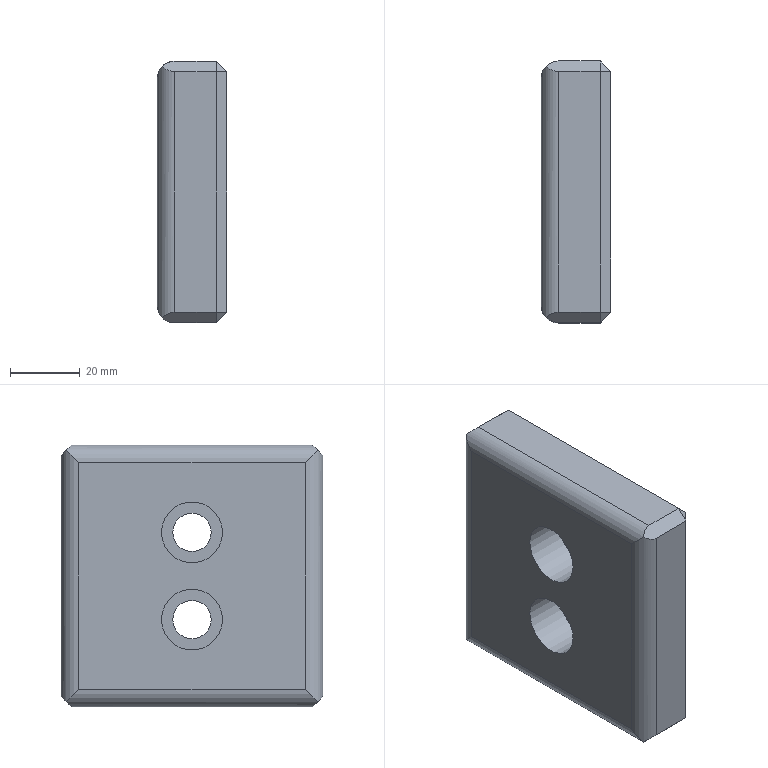Part | NX | features MAIN_BODY 2 | 1 solid | 28 faces | box 20 x 75 x 75 mm | volume 102061 mm3 | plane 20 | cylinder 8 | commonest cylinder face diameters 10 x4 11 x2 17.5 x2
STEP:
#1=CARTESIAN_POINT('',(-393.,34.5,70.));
#2=VERTEX_POINT('',#1);
#3=CARTESIAN_POINT('',(-405.,34.5,70.));
#4=VERTEX_POINT('',#3);
#5=CARTESIAN_POINT('',(-410.,34.5,70.));
#6=DIRECTION('',(-1.,0.,0.));
#7=VECTOR('',#6,1000.);
#8=LINE('',#5,#7);
#9=EDGE_CURVE('',#2,#4,#8,.T.);
#10=ORIENTED_EDGE('',*,*,#9,.T.);
#11=CARTESIAN_POINT('',(-405.,-34.5,70.));
#12=VERTEX_POINT('',#11);
#13=CARTESIAN_POINT('',(-405.,-34.5,70.));
#14=DIRECTION('',(0.,-1.,0.));
#15=VECTOR('',#14,1000.);
#16=LINE('',#13,#15);
#17=EDGE_CURVE('',#4,#12,#16,.T.);
#18=ORIENTED_EDGE('',*,*,#17,.T.);
#19=CARTESIAN_POINT('',(-393.,-34.5,70.));
#20=VERTEX_POINT('',#19);
#21=CARTESIAN_POINT('',(-410.,-34.5,70.));
#22=DIRECTION('',(1.,0.,0.));
#23=VECTOR('',#22,1000.);
#24=LINE('',#21,#23);
#25=EDGE_CURVE('',#12,#20,#24,.T.);
#26=ORIENTED_EDGE('',*,*,#25,.T.);
#27=CARTESIAN_POINT('',(-393.,37.5,70.));
#28=DIRECTION('',(0.,1.,0.));
#29=VECTOR('',#28,1000.);
#30=LINE('',#27,#29);
#31=EDGE_CURVE('',#20,#2,#30,.T.);
#32=ORIENTED_EDGE('',*,*,#31,.T.);
#33=EDGE_LOOP('',(#10,#18,#26,#32));
#34=FACE_BOUND('',#33,.T.);
#35=CARTESIAN_POINT('',(-410.,37.5,70.));
#36=DIRECTION('',(0.,0.,1.));
#37=DIRECTION('',(0.,1.,0.));
#38=AXIS2_PLACEMENT_3D('',#35,#36,#37);
#39=PLANE('',#38);
#40=ADVANCED_FACE('',(#34),#39,.T.);
#41=CARTESIAN_POINT('',(-393.,-37.5,67.));
#42=VERTEX_POINT('',#41);
#43=CARTESIAN_POINT('',(-405.,-37.5,67.));
#44=VERTEX_POINT('',#43);
#45=CARTESIAN_POINT('',(-410.,-37.5,67.));
#46=DIRECTION('',(-1.,0.,0.));
#47=VECTOR('',#46,1000.);
#48=LINE('',#45,#47);
#49=EDGE_CURVE('',#42,#44,#48,.T.);
#50=ORIENTED_EDGE('',*,*,#49,.T.);
#51=CARTESIAN_POINT('',(-405.,-37.5,-2.));
#52=VERTEX_POINT('',#51);
#53=CARTESIAN_POINT('',(-405.,-37.5,-2.));
#54=DIRECTION('',(0.,0.,-1.));
#55=VECTOR('',#54,1000.);
#56=LINE('',#53,#55);
#57=EDGE_CURVE('',#44,#52,#56,.T.);
#58=ORIENTED_EDGE('',*,*,#57,.T.);
#59=CARTESIAN_POINT('',(-393.,-37.5,-2.));
#60=VERTEX_POINT('',#59);
#61=CARTESIAN_POINT('',(-410.,-37.5,-2.));
#62=DIRECTION('',(1.,0.,0.));
#63=VECTOR('',#62,1000.);
#64=LINE('',#61,#63);
#65=EDGE_CURVE('',#52,#60,#64,.T.);
#66=ORIENTED_EDGE('',*,*,#65,.T.);
#67=CARTESIAN_POINT('',(-393.,-37.5,70.));
#68=DIRECTION('',(0.,0.,1.));
#69=VECTOR('',#68,1000.);
#70=LINE('',#67,#69);
#71=EDGE_CURVE('',#60,#42,#70,.T.);
#72=ORIENTED_EDGE('',*,*,#71,.T.);
#73=EDGE_LOOP('',(#50,#58,#66,#72));
#74=FACE_BOUND('',#73,.T.);
#75=CARTESIAN_POINT('',(-410.,-37.5,70.));
#76=DIRECTION('',(0.,-1.,0.));
#77=DIRECTION('',(0.,0.,1.));
#78=AXIS2_PLACEMENT_3D('',#75,#76,#77);
#79=PLANE('',#78);
#80=ADVANCED_FACE('',(#74),#79,.T.);
#81=CARTESIAN_POINT('',(-393.,-34.5,-5.));
#82=VERTEX_POINT('',#81);
#83=CARTESIAN_POINT('',(-405.,-34.5,-5.));
#84=VERTEX_POINT('',#83);
#85=CARTESIAN_POINT('',(-410.,-34.5,-5.));
#86=DIRECTION('',(-1.,0.,0.));
#87=VECTOR('',#86,1000.);
#88=LINE('',#85,#87);
#89=EDGE_CURVE('',#82,#84,#88,.T.);
#90=ORIENTED_EDGE('',*,*,#89,.T.);
#91=CARTESIAN_POINT('',(-405.,34.5,-5.));
#92=VERTEX_POINT('',#91);
#93=CARTESIAN_POINT('',(-405.,34.5,-5.));
#94=DIRECTION('',(0.,1.,0.));
#95=VECTOR('',#94,1000.);
#96=LINE('',#93,#95);
#97=EDGE_CURVE('',#84,#92,#96,.T.);
#98=ORIENTED_EDGE('',*,*,#97,.T.);
#99=CARTESIAN_POINT('',(-393.,34.5,-5.));
#100=VERTEX_POINT('',#99);
#101=CARTESIAN_POINT('',(-410.,34.5,-5.));
#102=DIRECTION('',(1.,0.,0.));
#103=VECTOR('',#102,1000.);
#104=LINE('',#101,#103);
#105=EDGE_CURVE('',#92,#100,#104,.T.);
#106=ORIENTED_EDGE('',*,*,#105,.T.);
#107=CARTESIAN_POINT('',(-393.,-37.5,-5.));
#108=DIRECTION('',(0.,-1.,0.));
#109=VECTOR('',#108,1000.);
#110=LINE('',#107,#109);
#111=EDGE_CURVE('',#100,#82,#110,.T.);
#112=ORIENTED_EDGE('',*,*,#111,.T.);
#113=EDGE_LOOP('',(#90,#98,#106,#112));
#114=FACE_BOUND('',#113,.T.);
#115=CARTESIAN_POINT('',(-410.,-37.5,-5.));
#116=DIRECTION('',(0.,0.,-1.));
#117=DIRECTION('',(-1.,0.,0.));
#118=AXIS2_PLACEMENT_3D('',#115,#116,#117);
#119=PLANE('',#118);
#120=ADVANCED_FACE('',(#114),#119,.T.);
#121=CARTESIAN_POINT('',(-393.,37.5,-2.));
#122=VERTEX_POINT('',#121);
#123=CARTESIAN_POINT('',(-405.,37.5,-2.));
#124=VERTEX_POINT('',#123);
#125=CARTESIAN_POINT('',(-410.,37.5,-2.));
#126=DIRECTION('',(-1.,0.,0.));
#127=VECTOR('',#126,1000.);
#128=LINE('',#125,#127);
#129=EDGE_CURVE('',#122,#124,#128,.T.);
#130=ORIENTED_EDGE('',*,*,#129,.T.);
#131=CARTESIAN_POINT('',(-405.,37.5,67.));
#132=VERTEX_POINT('',#131);
#133=CARTESIAN_POINT('',(-405.,37.5,67.));
#134=DIRECTION('',(0.,0.,1.));
#135=VECTOR('',#134,1000.);
#136=LINE('',#133,#135);
#137=EDGE_CURVE('',#124,#132,#136,.T.);
#138=ORIENTED_EDGE('',*,*,#137,.T.);
#139=CARTESIAN_POINT('',(-393.,37.5,67.));
#140=VERTEX_POINT('',#139);
#141=CARTESIAN_POINT('',(-410.,37.5,67.));
#142=DIRECTION('',(1.,0.,0.));
#143=VECTOR('',#142,1000.);
#144=LINE('',#141,#143);
#145=EDGE_CURVE('',#132,#140,#144,.T.);
#146=ORIENTED_EDGE('',*,*,#145,.T.);
#147=CARTESIAN_POINT('',(-393.,37.5,-5.));
#148=DIRECTION('',(0.,0.,-1.));
#149=VECTOR('',#148,1000.);
#150=LINE('',#147,#149);
#151=EDGE_CURVE('',#140,#122,#150,.T.);
#152=ORIENTED_EDGE('',*,*,#151,.T.);
#153=EDGE_LOOP('',(#130,#138,#146,#152));
#154=FACE_BOUND('',#153,.T.);
#155=CARTESIAN_POINT('',(-410.,37.5,-5.));
#156=DIRECTION('',(0.,1.,0.));
#157=DIRECTION('',(0.,0.,-1.));
#158=AXIS2_PLACEMENT_3D('',#155,#156,#157);
#159=PLANE('',#158);
#160=ADVANCED_FACE('',(#154),#159,.T.);
#161=CARTESIAN_POINT('',(-410.,-32.5,0.));
#162=VERTEX_POINT('',#161);
#163=CARTESIAN_POINT('',(-410.,-32.5,65.));
#164=VERTEX_POINT('',#163);
#165=CARTESIAN_POINT('',(-410.,-32.5,67.));
#166=DIRECTION('',(0.,0.,-1.));
#167=VECTOR('',#166,1000.);
#168=LINE('',#165,#167);
#169=EDGE_CURVE('',#162,#164,#168,.F.);
#170=ORIENTED_EDGE('',*,*,#169,.T.);
#171=CARTESIAN_POINT('',(-410.,32.5,65.));
#172=VERTEX_POINT('',#171);
#173=CARTESIAN_POINT('',(-410.,34.5,65.));
#174=DIRECTION('',(0.,-1.,0.));
#175=VECTOR('',#174,1000.);
#176=LINE('',#173,#175);
#177=EDGE_CURVE('',#164,#172,#176,.F.);
#178=ORIENTED_EDGE('',*,*,#177,.T.);
#179=CARTESIAN_POINT('',(-410.,32.5,0.));
#180=VERTEX_POINT('',#179);
#181=CARTESIAN_POINT('',(-410.,32.5,-2.));
#182=DIRECTION('',(0.,0.,1.));
#183=VECTOR('',#182,1000.);
#184=LINE('',#181,#183);
#185=EDGE_CURVE('',#172,#180,#184,.F.);
#186=ORIENTED_EDGE('',*,*,#185,.T.);
#187=CARTESIAN_POINT('',(-410.,-34.5,0.));
#188=DIRECTION('',(0.,1.,0.));
#189=VECTOR('',#188,1000.);
#190=LINE('',#187,#189);
#191=EDGE_CURVE('',#180,#162,#190,.F.);
#192=ORIENTED_EDGE('',*,*,#191,.T.);
#193=EDGE_LOOP('',(#170,#178,#186,#192));
#194=FACE_BOUND('',#193,.T.);
#195=CARTESIAN_POINT('',(-410.,-8.75,20.));
#196=VERTEX_POINT('',#195);
#197=CARTESIAN_POINT('',(-410.,0.,20.));
#198=DIRECTION('',(1.,0.,0.));
#199=DIRECTION('',(0.,-1.,0.));
#200=AXIS2_PLACEMENT_3D('',#197,#198,#199);
#201=CIRCLE('',#200,8.75);
#202=EDGE_CURVE('',#196,#196,#201,.T.);
#203=ORIENTED_EDGE('',*,*,#202,.T.);
#204=EDGE_LOOP('',(#203));
#205=FACE_BOUND('',#204,.T.);
#206=CARTESIAN_POINT('',(-410.,-8.75,45.));
#207=VERTEX_POINT('',#206);
#208=CARTESIAN_POINT('',(-410.,0.,45.));
#209=DIRECTION('',(1.,0.,0.));
#210=DIRECTION('',(0.,-1.,0.));
#211=AXIS2_PLACEMENT_3D('',#208,#209,#210);
#212=CIRCLE('',#211,8.75);
#213=EDGE_CURVE('',#207,#207,#212,.T.);
#214=ORIENTED_EDGE('',*,*,#213,.T.);
#215=EDGE_LOOP('',(#214));
#216=FACE_BOUND('',#215,.T.);
#217=CARTESIAN_POINT('',(-410.,-37.5,70.));
#218=DIRECTION('',(1.,0.,0.));
#219=DIRECTION('',(0.,-1.,0.));
#220=AXIS2_PLACEMENT_3D('',#217,#218,#219);
#221=PLANE('',#220);
#222=ADVANCED_FACE('',(#194,#205,#216),#221,.F.);
#223=CARTESIAN_POINT('',(-390.,34.5,67.));
#224=VERTEX_POINT('',#223);
#225=CARTESIAN_POINT('',(-390.,-34.5,67.));
#226=VERTEX_POINT('',#225);
#227=CARTESIAN_POINT('',(-390.,-37.5,67.));
#228=DIRECTION('',(0.,-1.,0.));
#229=VECTOR('',#228,1000.);
#230=LINE('',#227,#229);
#231=EDGE_CURVE('',#224,#226,#230,.T.);
#232=ORIENTED_EDGE('',*,*,#231,.T.);
#233=CARTESIAN_POINT('',(-390.,-34.5,-2.));
#234=VERTEX_POINT('',#233);
#235=CARTESIAN_POINT('',(-390.,-34.5,70.));
#236=DIRECTION('',(0.,0.,-1.));
#237=VECTOR('',#236,1000.);
#238=LINE('',#235,#237);
#239=EDGE_CURVE('',#226,#234,#238,.T.);
#240=ORIENTED_EDGE('',*,*,#239,.T.);
#241=CARTESIAN_POINT('',(-390.,34.5,-2.));
#242=VERTEX_POINT('',#241);
#243=CARTESIAN_POINT('',(-390.,-37.5,-2.));
#244=DIRECTION('',(0.,1.,0.));
#245=VECTOR('',#244,1000.);
#246=LINE('',#243,#245);
#247=EDGE_CURVE('',#234,#242,#246,.T.);
#248=ORIENTED_EDGE('',*,*,#247,.T.);
#249=CARTESIAN_POINT('',(-390.,34.5,70.));
#250=DIRECTION('',(0.,0.,1.));
#251=VECTOR('',#250,1000.);
#252=LINE('',#249,#251);
#253=EDGE_CURVE('',#242,#224,#252,.T.);
#254=ORIENTED_EDGE('',*,*,#253,.T.);
#255=EDGE_LOOP('',(#232,#240,#248,#254));
#256=FACE_BOUND('',#255,.T.);
#257=CARTESIAN_POINT('',(-390.,-5.5,20.));
#258=VERTEX_POINT('',#257);
#259=CARTESIAN_POINT('',(-390.,0.,20.));
#260=DIRECTION('',(1.,0.,0.));
#261=DIRECTION('',(0.,-1.,0.));
#262=AXIS2_PLACEMENT_3D('',#259,#260,#261);
#263=CIRCLE('',#262,5.5);
#264=EDGE_CURVE('',#258,#258,#263,.T.);
#265=ORIENTED_EDGE('',*,*,#264,.F.);
#266=EDGE_LOOP('',(#265));
#267=FACE_BOUND('',#266,.T.);
#268=CARTESIAN_POINT('',(-390.,-5.5,45.));
#269=VERTEX_POINT('',#268);
#270=CARTESIAN_POINT('',(-390.,0.,45.));
#271=DIRECTION('',(1.,0.,0.));
#272=DIRECTION('',(0.,-1.,0.));
#273=AXIS2_PLACEMENT_3D('',#270,#271,#272);
#274=CIRCLE('',#273,5.5);
#275=EDGE_CURVE('',#269,#269,#274,.T.);
#276=ORIENTED_EDGE('',*,*,#275,.F.);
#277=EDGE_LOOP('',(#276));
#278=FACE_BOUND('',#277,.T.);
#279=CARTESIAN_POINT('',(-390.,-37.5,70.));
#280=DIRECTION('',(1.,0.,0.));
#281=DIRECTION('',(0.,-1.,0.));
#282=AXIS2_PLACEMENT_3D('',#279,#280,#281);
#283=PLANE('',#282);
#284=ADVANCED_FACE('',(#256,#267,#278),#283,.T.);
#285=ORIENTED_EDGE('',*,*,#275,.T.);
#286=EDGE_LOOP('',(#285));
#287=FACE_BOUND('',#286,.T.);
#288=CARTESIAN_POINT('',(-398.,-5.5,45.));
#289=VERTEX_POINT('',#288);
#290=CARTESIAN_POINT('',(-398.,0.,45.));
#291=DIRECTION('',(1.,0.,0.));
#292=DIRECTION('',(0.,-1.,0.));
#293=AXIS2_PLACEMENT_3D('',#290,#291,#292);
#294=CIRCLE('',#293,5.5);
#295=EDGE_CURVE('',#289,#289,#294,.T.);
#296=ORIENTED_EDGE('',*,*,#295,.F.);
#297=EDGE_LOOP('',(#296));
#298=FACE_BOUND('',#297,.T.);
#299=CARTESIAN_POINT('',(-360.,0.,45.));
#300=DIRECTION('',(1.,0.,0.));
#301=DIRECTION('',(0.,-1.,0.));
#302=AXIS2_PLACEMENT_3D('',#299,#300,#301);
#303=CYLINDRICAL_SURFACE('',#302,5.5);
#304=ADVANCED_FACE('',(#287,#298),#303,.F.);
#305=ORIENTED_EDGE('',*,*,#295,.T.);
#306=EDGE_LOOP('',(#305));
#307=FACE_BOUND('',#306,.T.);
#308=CARTESIAN_POINT('',(-398.,-8.75,45.));
#309=VERTEX_POINT('',#308);
#310=CARTESIAN_POINT('',(-398.,0.,45.));
#311=DIRECTION('',(1.,0.,0.));
#312=DIRECTION('',(0.,-1.,0.));
#313=AXIS2_PLACEMENT_3D('',#310,#311,#312);
#314=CIRCLE('',#313,8.75);
#315=EDGE_CURVE('',#309,#309,#314,.T.);
#316=ORIENTED_EDGE('',*,*,#315,.F.);
#317=EDGE_LOOP('',(#316));
#318=FACE_BOUND('',#317,.T.);
#319=CARTESIAN_POINT('',(-398.,0.,45.));
#320=DIRECTION('',(1.,0.,0.));
#321=DIRECTION('',(0.,-1.,0.));
#322=AXIS2_PLACEMENT_3D('',#319,#320,#321);
#323=PLANE('',#322);
#324=ADVANCED_FACE('',(#307,#318),#323,.F.);
#325=ORIENTED_EDGE('',*,*,#315,.T.);
#326=EDGE_LOOP('',(#325));
#327=FACE_BOUND('',#326,.T.);
#328=ORIENTED_EDGE('',*,*,#213,.F.);
#329=EDGE_LOOP('',(#328));
#330=FACE_BOUND('',#329,.T.);
#331=CARTESIAN_POINT('',(-410.,0.,45.));
#332=DIRECTION('',(1.,0.,0.));
#333=DIRECTION('',(0.,-1.,0.));
#334=AXIS2_PLACEMENT_3D('',#331,#332,#333);
#335=CYLINDRICAL_SURFACE('',#334,8.75);
#336=ADVANCED_FACE('',(#327,#330),#335,.F.);
#337=ORIENTED_EDGE('',*,*,#264,.T.);
#338=EDGE_LOOP('',(#337));
#339=FACE_BOUND('',#338,.T.);
#340=CARTESIAN_POINT('',(-398.,-5.5,20.));
#341=VERTEX_POINT('',#340);
#342=CARTESIAN_POINT('',(-398.,0.,20.));
#343=DIRECTION('',(1.,0.,0.));
#344=DIRECTION('',(0.,-1.,0.));
#345=AXIS2_PLACEMENT_3D('',#342,#343,#344);
#346=CIRCLE('',#345,5.5);
#347=EDGE_CURVE('',#341,#341,#346,.T.);
#348=ORIENTED_EDGE('',*,*,#347,.F.);
#349=EDGE_LOOP('',(#348));
#350=FACE_BOUND('',#349,.T.);
#351=CARTESIAN_POINT('',(-360.,0.,20.));
#352=DIRECTION('',(1.,0.,0.));
#353=DIRECTION('',(0.,-1.,0.));
#354=AXIS2_PLACEMENT_3D('',#351,#352,#353);
#355=CYLINDRICAL_SURFACE('',#354,5.5);
#356=ADVANCED_FACE('',(#339,#350),#355,.F.);
#357=ORIENTED_EDGE('',*,*,#347,.T.);
#358=EDGE_LOOP('',(#357));
#359=FACE_BOUND('',#358,.T.);
#360=CARTESIAN_POINT('',(-398.,-8.75,20.));
#361=VERTEX_POINT('',#360);
#362=CARTESIAN_POINT('',(-398.,0.,20.));
#363=DIRECTION('',(1.,0.,0.));
#364=DIRECTION('',(0.,-1.,0.));
#365=AXIS2_PLACEMENT_3D('',#362,#363,#364);
#366=CIRCLE('',#365,8.75);
#367=EDGE_CURVE('',#361,#361,#366,.T.);
#368=ORIENTED_EDGE('',*,*,#367,.F.);
#369=EDGE_LOOP('',(#368));
#370=FACE_BOUND('',#369,.T.);
#371=CARTESIAN_POINT('',(-398.,0.,20.));
#372=DIRECTION('',(1.,0.,0.));
#373=DIRECTION('',(0.,-1.,0.));
#374=AXIS2_PLACEMENT_3D('',#371,#372,#373);
#375=PLANE('',#374);
#376=ADVANCED_FACE('',(#359,#370),#375,.F.);
#377=ORIENTED_EDGE('',*,*,#367,.T.);
#378=EDGE_LOOP('',(#377));
#379=FACE_BOUND('',#378,.T.);
#380=ORIENTED_EDGE('',*,*,#202,.F.);
#381=EDGE_LOOP('',(#380));
#382=FACE_BOUND('',#381,.T.);
#383=CARTESIAN_POINT('',(-410.,0.,20.));
#384=DIRECTION('',(1.,0.,0.));
#385=DIRECTION('',(0.,-1.,0.));
#386=AXIS2_PLACEMENT_3D('',#383,#384,#385);
#387=CYLINDRICAL_SURFACE('',#386,8.75);
#388=ADVANCED_FACE('',(#379,#382),#387,.F.);
#389=CARTESIAN_POINT('',(-408.571,36.,68.5));
#390=VERTEX_POINT('',#389);
#391=CARTESIAN_POINT('',(-405.,32.5,72.));
#392=DIRECTION('',(0.,-0.7071,-0.7071));
#393=DIRECTION('',(0.,0.7071,-0.7071));
#394=AXIS2_PLACEMENT_3D('',#391,#392,#393);
#395=ELLIPSE('',#394,7.071,5.);
#396=EDGE_CURVE('',#132,#390,#395,.F.);
#397=ORIENTED_EDGE('',*,*,#396,.T.);
#398=CARTESIAN_POINT('',(-405.,39.5,65.));
#399=DIRECTION('',(0.,-0.7071,-0.7071));
#400=DIRECTION('',(0.,0.7071,-0.7071));
#401=AXIS2_PLACEMENT_3D('',#398,#399,#400);
#402=ELLIPSE('',#401,7.071,5.);
#403=EDGE_CURVE('',#390,#4,#402,.F.);
#404=ORIENTED_EDGE('',*,*,#403,.T.);
#405=ORIENTED_EDGE('',*,*,#9,.F.);
#406=CARTESIAN_POINT('',(-393.,36.,68.5));
#407=DIRECTION('',(0.,0.7071,-0.7071));
#408=VECTOR('',#407,1000.);
#409=LINE('',#406,#408);
#410=EDGE_CURVE('',#140,#2,#409,.F.);
#411=ORIENTED_EDGE('',*,*,#410,.F.);
#412=ORIENTED_EDGE('',*,*,#145,.F.);
#413=EDGE_LOOP('',(#397,#404,#405,#411,#412));
#414=FACE_BOUND('',#413,.T.);
#415=CARTESIAN_POINT('',(-410.,37.5,67.));
#416=DIRECTION('',(0.,-0.7071,-0.7071));
#417=DIRECTION('',(0.,-0.7071,0.7071));
#418=AXIS2_PLACEMENT_3D('',#415,#416,#417);
#419=PLANE('',#418);
#420=ADVANCED_FACE('',(#414),#419,.F.);
#421=CARTESIAN_POINT('',(-390.,34.5,-2.));
#422=DIRECTION('',(-0.7071,0.7071,0.));
#423=VECTOR('',#422,1000.);
#424=LINE('',#421,#423);
#425=EDGE_CURVE('',#122,#242,#424,.F.);
#426=ORIENTED_EDGE('',*,*,#425,.F.);
#427=ORIENTED_EDGE('',*,*,#151,.F.);
#428=CARTESIAN_POINT('',(-390.,34.5,67.));
#429=DIRECTION('',(0.7071,-0.7071,0.));
#430=VECTOR('',#429,1000.);
#431=LINE('',#428,#430);
#432=EDGE_CURVE('',#224,#140,#431,.F.);
#433=ORIENTED_EDGE('',*,*,#432,.F.);
#434=ORIENTED_EDGE('',*,*,#253,.F.);
#435=EDGE_LOOP('',(#426,#427,#433,#434));
#436=FACE_BOUND('',#435,.T.);
#437=CARTESIAN_POINT('',(-390.,34.5,70.));
#438=DIRECTION('',(-0.7071,-0.7071,0.));
#439=DIRECTION('',(-0.7071,0.7071,0.));
#440=AXIS2_PLACEMENT_3D('',#437,#438,#439);
#441=PLANE('',#440);
#442=ADVANCED_FACE('',(#436),#441,.F.);
#443=ORIENTED_EDGE('',*,*,#105,.F.);
#444=CARTESIAN_POINT('',(-408.571,36.,-3.5));
#445=VERTEX_POINT('',#444);
#446=CARTESIAN_POINT('',(-405.,39.5,0.));
#447=DIRECTION('',(0.,-0.7071,0.7071));
#448=DIRECTION('',(0.,-0.7071,-0.7071));
#449=AXIS2_PLACEMENT_3D('',#446,#447,#448);
#450=ELLIPSE('',#449,7.071,5.);
#451=EDGE_CURVE('',#92,#445,#450,.F.);
#452=ORIENTED_EDGE('',*,*,#451,.T.);
#453=CARTESIAN_POINT('',(-405.,32.5,-7.));
#454=DIRECTION('',(0.,-0.7071,0.7071));
#455=DIRECTION('',(0.,-0.7071,-0.7071));
#456=AXIS2_PLACEMENT_3D('',#453,#454,#455);
#457=ELLIPSE('',#456,7.071,5.);
#458=EDGE_CURVE('',#445,#124,#457,.F.);
#459=ORIENTED_EDGE('',*,*,#458,.T.);
#460=ORIENTED_EDGE('',*,*,#129,.F.);
#461=CARTESIAN_POINT('',(-393.,36.,-3.5));
#462=DIRECTION('',(0.,-0.7071,-0.7071));
#463=VECTOR('',#462,1000.);
#464=LINE('',#461,#463);
#465=EDGE_CURVE('',#100,#122,#464,.F.);
#466=ORIENTED_EDGE('',*,*,#465,.F.);
#467=EDGE_LOOP('',(#443,#452,#459,#460,#466));
#468=FACE_BOUND('',#467,.T.);
#469=CARTESIAN_POINT('',(-410.,34.5,-5.));
#470=DIRECTION('',(0.,-0.7071,0.7071));
#471=DIRECTION('',(0.,0.7071,0.7071));
#472=AXIS2_PLACEMENT_3D('',#469,#470,#471);
#473=PLANE('',#472);
#474=ADVANCED_FACE('',(#468),#473,.F.);
#475=ORIENTED_EDGE('',*,*,#432,.T.);
#476=ORIENTED_EDGE('',*,*,#410,.T.);
#477=CARTESIAN_POINT('',(-390.,34.5,67.));
#478=DIRECTION('',(-0.7071,0.,0.7071));
#479=VECTOR('',#478,1000.);
#480=LINE('',#477,#479);
#481=EDGE_CURVE('',#224,#2,#480,.T.);
#482=ORIENTED_EDGE('',*,*,#481,.F.);
#483=EDGE_LOOP('',(#475,#476,#482));
#484=FACE_BOUND('',#483,.T.);
#485=CARTESIAN_POINT('',(-390.,34.5,67.));
#486=DIRECTION('',(0.5774,0.5774,0.5774));
#487=DIRECTION('',(0.7071,-0.7071,0.));
#488=AXIS2_PLACEMENT_3D('',#485,#486,#487);
#489=PLANE('',#488);
#490=ADVANCED_FACE('',(#484),#489,.T.);
#491=ORIENTED_EDGE('',*,*,#465,.T.);
#492=ORIENTED_EDGE('',*,*,#425,.T.);
#493=CARTESIAN_POINT('',(-390.,34.5,-2.));
#494=DIRECTION('',(0.7071,0.,0.7071));
#495=VECTOR('',#494,1000.);
#496=LINE('',#493,#495);
#497=EDGE_CURVE('',#100,#242,#496,.T.);
#498=ORIENTED_EDGE('',*,*,#497,.F.);
#499=EDGE_LOOP('',(#491,#492,#498));
#500=FACE_BOUND('',#499,.T.);
#501=CARTESIAN_POINT('',(-390.,34.5,-2.));
#502=DIRECTION('',(0.5774,0.5774,-0.5774));
#503=DIRECTION('',(0.7071,-0.7071,0.));
#504=AXIS2_PLACEMENT_3D('',#501,#502,#503);
#505=PLANE('',#504);
#506=ADVANCED_FACE('',(#500),#505,.T.);
#507=ORIENTED_EDGE('',*,*,#25,.F.);
#508=CARTESIAN_POINT('',(-408.571,-36.,68.5));
#509=VERTEX_POINT('',#508);
#510=CARTESIAN_POINT('',(-405.,-39.5,65.));
#511=DIRECTION('',(0.,0.7071,-0.7071));
#512=DIRECTION('',(0.,0.7071,0.7071));
#513=AXIS2_PLACEMENT_3D('',#510,#511,#512);
#514=ELLIPSE('',#513,7.071,5.);
#515=EDGE_CURVE('',#12,#509,#514,.F.);
#516=ORIENTED_EDGE('',*,*,#515,.T.);
#517=CARTESIAN_POINT('',(-405.,-32.5,72.));
#518=DIRECTION('',(0.,0.7071,-0.7071));
#519=DIRECTION('',(0.,0.7071,0.7071));
#520=AXIS2_PLACEMENT_3D('',#517,#518,#519);
#521=ELLIPSE('',#520,7.071,5.);
#522=EDGE_CURVE('',#509,#44,#521,.F.);
#523=ORIENTED_EDGE('',*,*,#522,.T.);
#524=ORIENTED_EDGE('',*,*,#49,.F.);
#525=CARTESIAN_POINT('',(-393.,-37.5,67.));
#526=DIRECTION('',(0.,0.7071,0.7071));
#527=VECTOR('',#526,1000.);
#528=LINE('',#525,#527);
#529=EDGE_CURVE('',#20,#42,#528,.F.);
#530=ORIENTED_EDGE('',*,*,#529,.F.);
#531=EDGE_LOOP('',(#507,#516,#523,#524,#530));
#532=FACE_BOUND('',#531,.T.);
#533=CARTESIAN_POINT('',(-410.,-34.5,70.));
#534=DIRECTION('',(0.,0.7071,-0.7071));
#535=DIRECTION('',(0.,-0.7071,-0.7071));
#536=AXIS2_PLACEMENT_3D('',#533,#534,#535);
#537=PLANE('',#536);
#538=ADVANCED_FACE('',(#532),#537,.F.);
#539=ORIENTED_EDGE('',*,*,#481,.T.);
#540=ORIENTED_EDGE('',*,*,#31,.F.);
#541=CARTESIAN_POINT('',(-391.5,-34.5,68.5));
#542=DIRECTION('',(0.7071,0.,-0.7071));
#543=VECTOR('',#542,1000.);
#544=LINE('',#541,#543);
#545=EDGE_CURVE('',#226,#20,#544,.F.);
#546=ORIENTED_EDGE('',*,*,#545,.F.);
#547=ORIENTED_EDGE('',*,*,#231,.F.);
#548=EDGE_LOOP('',(#539,#540,#546,#547));
#549=FACE_BOUND('',#548,.T.);
#550=CARTESIAN_POINT('',(-390.,-37.5,67.));
#551=DIRECTION('',(-0.7071,0.,-0.7071));
#552=DIRECTION('',(-0.7071,0.,0.7071));
#553=AXIS2_PLACEMENT_3D('',#550,#551,#552);
#554=PLANE('',#553);
#555=ADVANCED_FACE('',(#549),#554,.F.);
#556=ORIENTED_EDGE('',*,*,#497,.T.);
#557=ORIENTED_EDGE('',*,*,#247,.F.);
#558=CARTESIAN_POINT('',(-390.,-34.5,-2.));
#559=DIRECTION('',(-0.7071,0.,-0.7071));
#560=VECTOR('',#559,1000.);
#561=LINE('',#558,#560);
#562=EDGE_CURVE('',#82,#234,#561,.F.);
#563=ORIENTED_EDGE('',*,*,#562,.F.);
#564=ORIENTED_EDGE('',*,*,#111,.F.);
#565=EDGE_LOOP('',(#556,#557,#563,#564));
#566=FACE_BOUND('',#565,.T.);
#567=CARTESIAN_POINT('',(-390.,-37.5,-2.));
#568=DIRECTION('',(-0.7071,0.,0.7071));
#569=DIRECTION('',(0.7071,0.,0.7071));
#570=AXIS2_PLACEMENT_3D('',#567,#568,#569);
#571=PLANE('',#570);
#572=ADVANCED_FACE('',(#566),#571,.F.);
#573=ORIENTED_EDGE('',*,*,#65,.F.);
#574=CARTESIAN_POINT('',(-408.571,-36.,-3.5));
#575=VERTEX_POINT('',#574);
#576=CARTESIAN_POINT('',(-405.,-32.5,-7.));
#577=DIRECTION('',(0.,0.7071,0.7071));
#578=DIRECTION('',(0.,-0.7071,0.7071));
#579=AXIS2_PLACEMENT_3D('',#576,#577,#578);
#580=ELLIPSE('',#579,7.071,5.);
#581=EDGE_CURVE('',#52,#575,#580,.F.);
#582=ORIENTED_EDGE('',*,*,#581,.T.);
#583=CARTESIAN_POINT('',(-405.,-39.5,0.));
#584=DIRECTION('',(0.,0.7071,0.7071));
#585=DIRECTION('',(0.,-0.7071,0.7071));
#586=AXIS2_PLACEMENT_3D('',#583,#584,#585);
#587=ELLIPSE('',#586,7.071,5.);
#588=EDGE_CURVE('',#575,#84,#587,.F.);
#589=ORIENTED_EDGE('',*,*,#588,.T.);
#590=ORIENTED_EDGE('',*,*,#89,.F.);
#591=CARTESIAN_POINT('',(-393.,-36.,-3.5));
#592=DIRECTION('',(0.,-0.7071,0.7071));
#593=VECTOR('',#592,1000.);
#594=LINE('',#591,#593);
#595=EDGE_CURVE('',#60,#82,#594,.F.);
#596=ORIENTED_EDGE('',*,*,#595,.F.);
#597=EDGE_LOOP('',(#573,#582,#589,#590,#596));
#598=FACE_BOUND('',#597,.T.);
#599=CARTESIAN_POINT('',(-410.,-37.5,-2.));
#600=DIRECTION('',(0.,0.7071,0.7071));
#601=DIRECTION('',(0.,0.7071,-0.7071));
#602=AXIS2_PLACEMENT_3D('',#599,#600,#601);
#603=PLANE('',#602);
#604=ADVANCED_FACE('',(#598),#603,.F.);
#605=ORIENTED_EDGE('',*,*,#545,.T.);
#606=ORIENTED_EDGE('',*,*,#529,.T.);
#607=CARTESIAN_POINT('',(-393.,-37.5,67.));
#608=DIRECTION('',(-0.7071,-0.7071,0.));
#609=VECTOR('',#608,1000.);
#610=LINE('',#607,#609);
#611=EDGE_CURVE('',#226,#42,#610,.T.);
#612=ORIENTED_EDGE('',*,*,#611,.F.);
#613=EDGE_LOOP('',(#605,#606,#612));
#614=FACE_BOUND('',#613,.T.);
#615=CARTESIAN_POINT('',(-393.,-37.5,67.));
#616=DIRECTION('',(0.5774,-0.5774,0.5774));
#617=DIRECTION('',(-0.7071,-0.7071,0.));
#618=AXIS2_PLACEMENT_3D('',#615,#616,#617);
#619=PLANE('',#618);
#620=ADVANCED_FACE('',(#614),#619,.T.);
#621=ORIENTED_EDGE('',*,*,#595,.T.);
#622=ORIENTED_EDGE('',*,*,#562,.T.);
#623=CARTESIAN_POINT('',(-390.,-34.5,-2.));
#624=DIRECTION('',(0.7071,0.7071,0.));
#625=VECTOR('',#624,1000.);
#626=LINE('',#623,#625);
#627=EDGE_CURVE('',#60,#234,#626,.T.);
#628=ORIENTED_EDGE('',*,*,#627,.F.);
#629=EDGE_LOOP('',(#621,#622,#628));
#630=FACE_BOUND('',#629,.T.);
#631=CARTESIAN_POINT('',(-390.,-34.5,-2.));
#632=DIRECTION('',(0.5774,-0.5774,-0.5774));
#633=DIRECTION('',(-0.7071,-0.7071,0.));
#634=AXIS2_PLACEMENT_3D('',#631,#632,#633);
#635=PLANE('',#634);
#636=ADVANCED_FACE('',(#630),#635,.T.);
#637=ORIENTED_EDGE('',*,*,#611,.T.);
#638=ORIENTED_EDGE('',*,*,#71,.F.);
#639=ORIENTED_EDGE('',*,*,#627,.T.);
#640=ORIENTED_EDGE('',*,*,#239,.F.);
#641=EDGE_LOOP('',(#637,#638,#639,#640));
#642=FACE_BOUND('',#641,.T.);
#643=CARTESIAN_POINT('',(-390.,-34.5,70.));
#644=DIRECTION('',(-0.7071,0.7071,0.));
#645=DIRECTION('',(0.7071,0.7071,0.));
#646=AXIS2_PLACEMENT_3D('',#643,#644,#645);
#647=PLANE('',#646);
#648=ADVANCED_FACE('',(#642),#647,.F.);
#649=CARTESIAN_POINT('',(-405.,-32.5,0.));
#650=DIRECTION('',(0.,-0.7071,0.7071));
#651=DIRECTION('',(0.,0.7071,0.7071));
#652=AXIS2_PLACEMENT_3D('',#649,#650,#651);
#653=ELLIPSE('',#652,7.071,5.);
#654=EDGE_CURVE('',#162,#575,#653,.T.);
#655=ORIENTED_EDGE('',*,*,#654,.F.);
#656=ORIENTED_EDGE('',*,*,#191,.F.);
#657=CARTESIAN_POINT('',(-405.,32.5,0.));
#658=DIRECTION('',(0.,-0.7071,-0.7071));
#659=DIRECTION('',(0.,-0.7071,0.7071));
#660=AXIS2_PLACEMENT_3D('',#657,#658,#659);
#661=ELLIPSE('',#660,7.071,5.);
#662=EDGE_CURVE('',#445,#180,#661,.F.);
#663=ORIENTED_EDGE('',*,*,#662,.F.);
#664=ORIENTED_EDGE('',*,*,#451,.F.);
#665=ORIENTED_EDGE('',*,*,#97,.F.);
#666=ORIENTED_EDGE('',*,*,#588,.F.);
#667=EDGE_LOOP('',(#655,#656,#663,#664,#665,#666));
#668=FACE_BOUND('',#667,.T.);
#669=CARTESIAN_POINT('',(-405.,-37.5,0.));
#670=DIRECTION('',(0.,-1.,0.));
#671=DIRECTION('',(-1.,0.,0.));
#672=AXIS2_PLACEMENT_3D('',#669,#670,#671);
#673=CYLINDRICAL_SURFACE('',#672,5.);
#674=ADVANCED_FACE('',(#668),#673,.T.);
#675=ORIENTED_EDGE('',*,*,#662,.T.);
#676=ORIENTED_EDGE('',*,*,#185,.F.);
#677=CARTESIAN_POINT('',(-405.,32.5,65.));
#678=DIRECTION('',(0.,0.7071,-0.7071));
#679=DIRECTION('',(0.,-0.7071,-0.7071));
#680=AXIS2_PLACEMENT_3D('',#677,#678,#679);
#681=ELLIPSE('',#680,7.071,5.);
#682=EDGE_CURVE('',#390,#172,#681,.F.);
#683=ORIENTED_EDGE('',*,*,#682,.F.);
#684=ORIENTED_EDGE('',*,*,#396,.F.);
#685=ORIENTED_EDGE('',*,*,#137,.F.);
#686=ORIENTED_EDGE('',*,*,#458,.F.);
#687=EDGE_LOOP('',(#675,#676,#683,#684,#685,#686));
#688=FACE_BOUND('',#687,.T.);
#689=CARTESIAN_POINT('',(-405.,32.5,-5.));
#690=DIRECTION('',(0.,0.,-1.));
#691=DIRECTION('',(0.,-1.,0.));
#692=AXIS2_PLACEMENT_3D('',#689,#690,#691);
#693=CYLINDRICAL_SURFACE('',#692,5.);
#694=ADVANCED_FACE('',(#688),#693,.T.);
#695=ORIENTED_EDGE('',*,*,#57,.F.);
#696=ORIENTED_EDGE('',*,*,#522,.F.);
#697=CARTESIAN_POINT('',(-405.,-32.5,65.));
#698=DIRECTION('',(0.,0.7071,0.7071));
#699=DIRECTION('',(0.,0.7071,-0.7071));
#700=AXIS2_PLACEMENT_3D('',#697,#698,#699);
#701=ELLIPSE('',#700,7.071,5.);
#702=EDGE_CURVE('',#164,#509,#701,.T.);
#703=ORIENTED_EDGE('',*,*,#702,.F.);
#704=ORIENTED_EDGE('',*,*,#169,.F.);
#705=ORIENTED_EDGE('',*,*,#654,.T.);
#706=ORIENTED_EDGE('',*,*,#581,.F.);
#707=EDGE_LOOP('',(#695,#696,#703,#704,#705,#706));
#708=FACE_BOUND('',#707,.T.);
#709=CARTESIAN_POINT('',(-405.,-32.5,70.));
#710=DIRECTION('',(0.,0.,1.));
#711=DIRECTION('',(0.,1.,0.));
#712=AXIS2_PLACEMENT_3D('',#709,#710,#711);
#713=CYLINDRICAL_SURFACE('',#712,5.);
#714=ADVANCED_FACE('',(#708),#713,.T.);
#715=ORIENTED_EDGE('',*,*,#682,.T.);
#716=ORIENTED_EDGE('',*,*,#177,.F.);
#717=ORIENTED_EDGE('',*,*,#702,.T.);
#718=ORIENTED_EDGE('',*,*,#515,.F.);
#719=ORIENTED_EDGE('',*,*,#17,.F.);
#720=ORIENTED_EDGE('',*,*,#403,.F.);
#721=EDGE_LOOP('',(#715,#716,#717,#718,#719,#720));
#722=FACE_BOUND('',#721,.T.);
#723=CARTESIAN_POINT('',(-405.,37.5,65.));
#724=DIRECTION('',(0.,1.,0.));
#725=DIRECTION('',(0.,0.,-1.));
#726=AXIS2_PLACEMENT_3D('',#723,#724,#725);
#727=CYLINDRICAL_SURFACE('',#726,5.);
#728=ADVANCED_FACE('',(#722),#727,.T.);
#729=CLOSED_SHELL('',(#40,#80,#120,#160,#222,#284,#304,#324,#336,#356,#376,#388,#420,#442,#474,#490,#506,#538,#555,#572,#604,#620,#636,#648,#674,#694,#714,#728));
#730=MANIFOLD_SOLID_BREP('',#729);
#731=(LENGTH_UNIT()NAMED_UNIT(*)SI_UNIT(.MILLI.,.METRE.));
#732=UNCERTAINTY_MEASURE_WITH_UNIT(LENGTH_MEASURE(0.00001),#731,'','');
#733=(NAMED_UNIT(*)PLANE_ANGLE_UNIT()SI_UNIT($,.RADIAN.));
#734=(NAMED_UNIT(*)SI_UNIT($,.STERADIAN.)SOLID_ANGLE_UNIT());
#735=(GEOMETRIC_REPRESENTATION_CONTEXT(3)GLOBAL_UNCERTAINTY_ASSIGNED_CONTEXT((#732))GLOBAL_UNIT_ASSIGNED_CONTEXT((#731,#733,#734))REPRESENTATION_CONTEXT('',''));
#736=ADVANCED_BREP_SHAPE_REPRESENTATION('',(#730),#735);